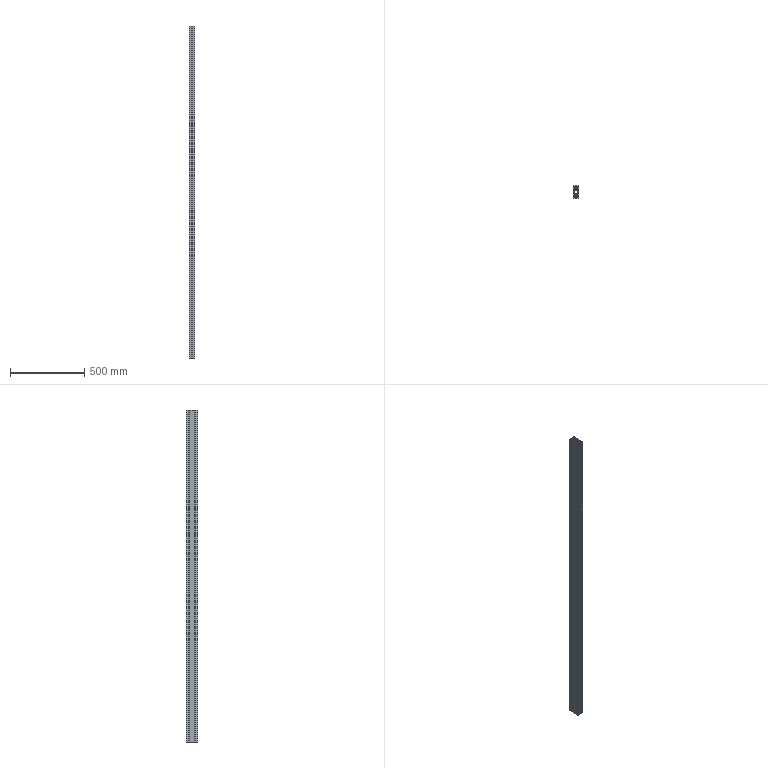Part | STEP file | 1.6米HFS8-4080-3000 | 1 solid | 170 faces | box 40 x 80 x 2230 mm | volume 2325189 mm3 | plane 112 | cylinder 58 | commonest cylinder face diameters 2 x44 10.5 x10 6 x4